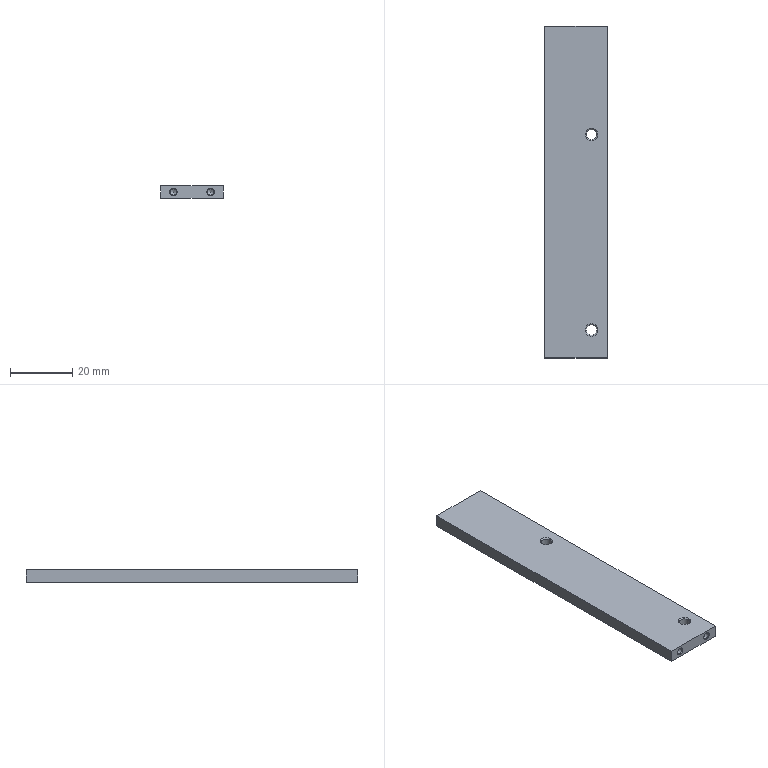Part | STEP file | Power mounting plate | 1 solid | 24 faces | box 20 x 107 x 4 mm | volume 8429 mm3 | cone 12 | plane 6 | cylinder 6 | commonest cylinder face diameters 1.6 x2 2.05 x2 3.3 x2